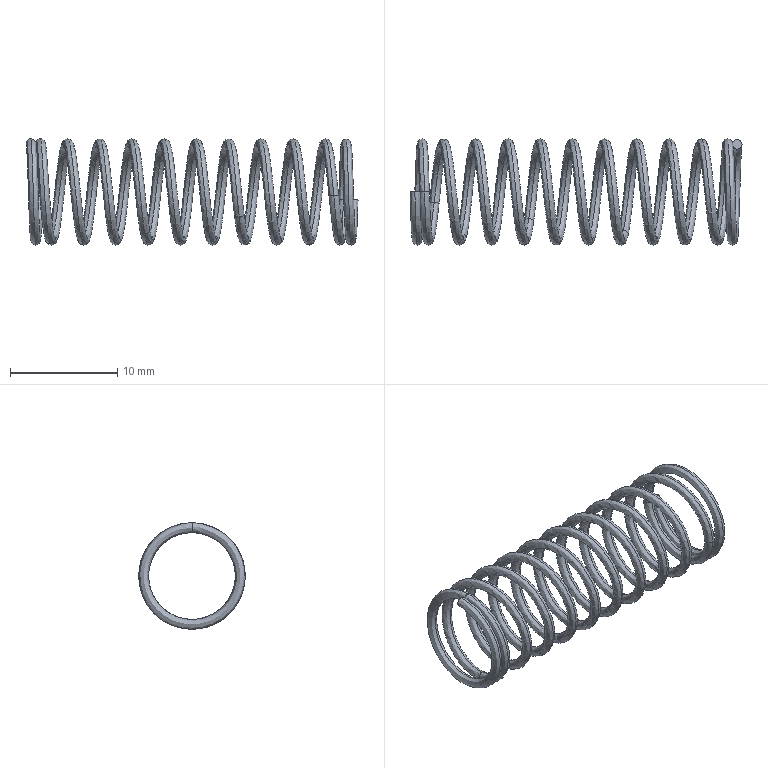Part | NX | features solid 2 | 1 solid | 16 faces | box 30.9 x 9.9 x 9.9 mm | volume 210.54 mm3 | spline 14 | plane 2